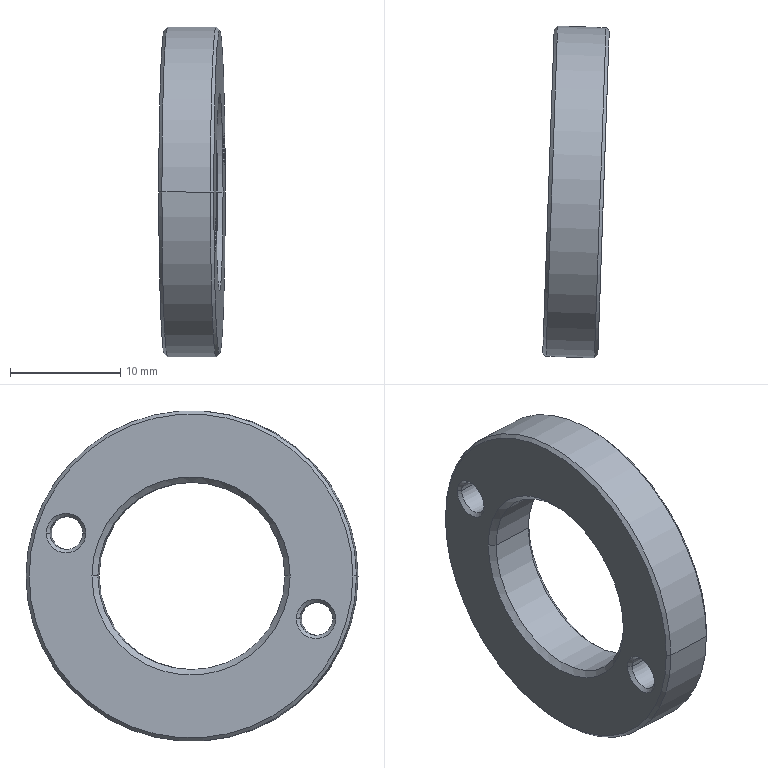Part | SolidWorks | features BaseBody 1 | 1 solid | 22 faces | box 6.032 x 30.136 x 30 mm | volume 2306 mm3 | cone 12 | cylinder 8 | plane 2 | commonest cylinder face diameters 3 x4 17 x2 30 x2
STEP:
#1=CARTESIAN_POINT('',(719.231,30.003,4.092));
#2=VERTEX_POINT('',#1);
#3=CARTESIAN_POINT('',(719.83,46.992,4.092));
#4=VERTEX_POINT('',#3);
#5=CARTESIAN_POINT('',(719.531,38.498,4.092));
#6=DIRECTION('',(0.9994,-0.0352,-0.000000013));
#7=DIRECTION('',(0.000000013,-0.000000004,1.));
#8=AXIS2_PLACEMENT_3D('',#5,#6,#7);
#9=CIRCLE('',#8,8.5);
#10=EDGE_CURVE('',#2,#4,#9,.T.);
#11=ORIENTED_EDGE('',*,*,#10,.F.);
#12=CARTESIAN_POINT('',(719.713,29.486,4.092));
#13=VERTEX_POINT('',#12);
#14=CARTESIAN_POINT('',(719.713,29.486,4.092));
#15=DIRECTION('',(0.6818,-0.7316,-0.000000009));
#16=VECTOR('',#15,1000.);
#17=LINE('',#14,#16);
#18=EDGE_CURVE('',#2,#13,#17,.T.);
#19=ORIENTED_EDGE('',*,*,#18,.T.);
#20=CARTESIAN_POINT('',(720.347,47.475,4.092));
#21=VERTEX_POINT('',#20);
#22=CARTESIAN_POINT('',(720.03,38.48,4.092));
#23=DIRECTION('',(0.9994,-0.0352,-0.000000013));
#24=DIRECTION('',(0.0352,0.9994,0.));
#25=AXIS2_PLACEMENT_3D('',#22,#23,#24);
#26=CIRCLE('',#25,9.);
#27=EDGE_CURVE('',#13,#21,#26,.T.);
#28=ORIENTED_EDGE('',*,*,#27,.T.);
#29=CARTESIAN_POINT('',(720.347,47.475,4.092));
#30=DIRECTION('',(0.7316,0.6818,-0.000000009));
#31=VECTOR('',#30,1000.);
#32=LINE('',#29,#31);
#33=EDGE_CURVE('',#4,#21,#32,.T.);
#34=ORIENTED_EDGE('',*,*,#33,.F.);
#35=EDGE_LOOP('',(#11,#19,#28,#34));
#36=FACE_OUTER_BOUND('',#35,.T.);
#37=CARTESIAN_POINT('',(720.03,38.48,4.092));
#38=DIRECTION('',(0.9994,-0.0352,-0.000000013));
#39=DIRECTION('',(0.0352,0.9994,0.));
#40=AXIS2_PLACEMENT_3D('',#37,#38,#39);
#41=CONICAL_SURFACE('',#40,9.,0.7854);
#42=ADVANCED_FACE('',(#36),#41,.F.);
#43=CARTESIAN_POINT('',(720.377,48.325,7.984));
#44=VERTEX_POINT('',#43);
#45=CARTESIAN_POINT('',(720.483,51.323,7.984));
#46=VERTEX_POINT('',#45);
#47=CARTESIAN_POINT('',(720.43,49.824,7.984));
#48=DIRECTION('',(0.9994,-0.0352,-0.000000013));
#49=DIRECTION('',(-0.0352,-0.9994,0.));
#50=AXIS2_PLACEMENT_3D('',#47,#48,#49);
#51=CIRCLE('',#50,1.5);
#52=EDGE_CURVE('',#44,#46,#51,.T.);
#53=ORIENTED_EDGE('',*,*,#52,.T.);
#54=CARTESIAN_POINT('',(715.786,51.489,7.984));
#55=VERTEX_POINT('',#54);
#56=CARTESIAN_POINT('',(715.486,51.499,7.984));
#57=DIRECTION('',(-0.9994,0.0352,0.000000013));
#58=VECTOR('',#57,1000.);
#59=LINE('',#56,#58);
#60=EDGE_CURVE('',#46,#55,#59,.T.);
#61=ORIENTED_EDGE('',*,*,#60,.T.);
#62=CARTESIAN_POINT('',(715.68,48.491,7.984));
#63=VERTEX_POINT('',#62);
#64=CARTESIAN_POINT('',(715.733,49.99,7.984));
#65=DIRECTION('',(0.9994,-0.0352,-0.000000013));
#66=DIRECTION('',(-0.0352,-0.9994,0.));
#67=AXIS2_PLACEMENT_3D('',#64,#65,#66);
#68=CIRCLE('',#67,1.5);
#69=EDGE_CURVE('',#63,#55,#68,.T.);
#70=ORIENTED_EDGE('',*,*,#69,.F.);
#71=CARTESIAN_POINT('',(715.38,48.501,7.984));
#72=DIRECTION('',(-0.9994,0.0352,0.000000013));
#73=VECTOR('',#72,1000.);
#74=LINE('',#71,#73);
#75=EDGE_CURVE('',#44,#63,#74,.T.);
#76=ORIENTED_EDGE('',*,*,#75,.F.);
#77=EDGE_LOOP('',(#53,#61,#70,#76));
#78=FACE_OUTER_BOUND('',#77,.T.);
#79=CARTESIAN_POINT('',(715.433,50.,7.984));
#80=DIRECTION('',(-0.9994,0.0352,0.000000013));
#81=DIRECTION('',(-0.0352,-0.9994,0.));
#82=AXIS2_PLACEMENT_3D('',#79,#80,#81);
#83=CYLINDRICAL_SURFACE('',#82,1.5);
#84=ADVANCED_FACE('',(#78),#83,.F.);
#85=CARTESIAN_POINT('',(719.578,25.637,0.1995));
#86=VERTEX_POINT('',#85);
#87=CARTESIAN_POINT('',(719.684,28.635,0.1995));
#88=VERTEX_POINT('',#87);
#89=CARTESIAN_POINT('',(719.631,27.136,0.1995));
#90=DIRECTION('',(0.9994,-0.0352,-0.000000013));
#91=DIRECTION('',(-0.0352,-0.9994,0.));
#92=AXIS2_PLACEMENT_3D('',#89,#90,#91);
#93=CIRCLE('',#92,1.5);
#94=EDGE_CURVE('',#86,#88,#93,.T.);
#95=ORIENTED_EDGE('',*,*,#94,.T.);
#96=CARTESIAN_POINT('',(714.986,28.8,0.1995));
#97=VERTEX_POINT('',#96);
#98=CARTESIAN_POINT('',(714.687,28.811,0.1995));
#99=DIRECTION('',(-0.9994,0.0352,0.000000013));
#100=VECTOR('',#99,1000.);
#101=LINE('',#98,#100);
#102=EDGE_CURVE('',#88,#97,#101,.T.);
#103=ORIENTED_EDGE('',*,*,#102,.T.);
#104=CARTESIAN_POINT('',(714.881,25.802,0.1995));
#105=VERTEX_POINT('',#104);
#106=CARTESIAN_POINT('',(714.934,27.301,0.1995));
#107=DIRECTION('',(0.9994,-0.0352,-0.000000013));
#108=DIRECTION('',(-0.0352,-0.9994,0.));
#109=AXIS2_PLACEMENT_3D('',#106,#107,#108);
#110=CIRCLE('',#109,1.5);
#111=EDGE_CURVE('',#105,#97,#110,.T.);
#112=ORIENTED_EDGE('',*,*,#111,.F.);
#113=CARTESIAN_POINT('',(714.581,25.813,0.1995));
#114=DIRECTION('',(-0.9994,0.0352,0.000000013));
#115=VECTOR('',#114,1000.);
#116=LINE('',#113,#115);
#117=EDGE_CURVE('',#86,#105,#116,.T.);
#118=ORIENTED_EDGE('',*,*,#117,.F.);
#119=EDGE_LOOP('',(#95,#103,#112,#118));
#120=FACE_OUTER_BOUND('',#119,.T.);
#121=CARTESIAN_POINT('',(714.634,27.312,0.1995));
#122=DIRECTION('',(-0.9994,0.0352,0.000000013));
#123=DIRECTION('',(-0.0352,-0.9994,0.));
#124=AXIS2_PLACEMENT_3D('',#121,#122,#123);
#125=CYLINDRICAL_SURFACE('',#124,1.5);
#126=ADVANCED_FACE('',(#120),#125,.F.);
#127=CARTESIAN_POINT('',(719.513,23.789,4.092));
#128=VERTEX_POINT('',#127);
#129=CARTESIAN_POINT('',(720.548,53.171,4.092));
#130=VERTEX_POINT('',#129);
#131=CARTESIAN_POINT('',(720.03,38.48,4.092));
#132=DIRECTION('',(-0.9994,0.0352,0.000000013));
#133=DIRECTION('',(-0.0352,-0.9994,0.));
#134=AXIS2_PLACEMENT_3D('',#131,#132,#133);
#135=CIRCLE('',#134,14.7);
#136=EDGE_CURVE('',#128,#130,#135,.T.);
#137=ORIENTED_EDGE('',*,*,#136,.T.);
#138=CARTESIAN_POINT('',(720.259,53.481,4.092));
#139=VERTEX_POINT('',#138);
#140=CARTESIAN_POINT('',(720.259,53.481,4.092));
#141=DIRECTION('',(-0.6818,0.7316,0.000000009));
#142=VECTOR('',#141,1000.);
#143=LINE('',#140,#142);
#144=EDGE_CURVE('',#130,#139,#143,.T.);
#145=ORIENTED_EDGE('',*,*,#144,.T.);
#146=CARTESIAN_POINT('',(719.202,23.5,4.092));
#147=VERTEX_POINT('',#146);
#148=CARTESIAN_POINT('',(719.731,38.491,4.092));
#149=DIRECTION('',(0.9994,-0.0352,-0.000000013));
#150=DIRECTION('',(0.000000013,-0.000000004,1.));
#151=AXIS2_PLACEMENT_3D('',#148,#149,#150);
#152=CIRCLE('',#151,15.);
#153=EDGE_CURVE('',#139,#147,#152,.T.);
#154=ORIENTED_EDGE('',*,*,#153,.T.);
#155=CARTESIAN_POINT('',(719.202,23.5,4.092));
#156=DIRECTION('',(-0.7316,-0.6818,0.000000009));
#157=VECTOR('',#156,1000.);
#158=LINE('',#155,#157);
#159=EDGE_CURVE('',#128,#147,#158,.T.);
#160=ORIENTED_EDGE('',*,*,#159,.F.);
#161=EDGE_LOOP('',(#137,#145,#154,#160));
#162=FACE_OUTER_BOUND('',#161,.T.);
#163=CARTESIAN_POINT('',(719.731,38.491,4.092));
#164=DIRECTION('',(-0.9994,0.0352,0.000000013));
#165=DIRECTION('',(-0.0352,-0.9994,0.));
#166=AXIS2_PLACEMENT_3D('',#163,#164,#165);
#167=CONICAL_SURFACE('',#166,15.,0.7854);
#168=ADVANCED_FACE('',(#162),#167,.T.);
#169=CARTESIAN_POINT('',(715.234,30.144,4.092));
#170=VERTEX_POINT('',#169);
#171=CARTESIAN_POINT('',(715.832,47.133,4.092));
#172=VERTEX_POINT('',#171);
#173=CARTESIAN_POINT('',(715.533,38.639,4.092));
#174=DIRECTION('',(0.9994,-0.0352,-0.000000013));
#175=DIRECTION('',(0.0352,0.9994,0.));
#176=AXIS2_PLACEMENT_3D('',#173,#174,#175);
#177=CIRCLE('',#176,8.5);
#178=EDGE_CURVE('',#170,#172,#177,.T.);
#179=ORIENTED_EDGE('',*,*,#178,.F.);
#180=CARTESIAN_POINT('',(717.233,30.073,4.092));
#181=DIRECTION('',(0.9994,-0.0352,-0.000000013));
#182=VECTOR('',#181,1000.);
#183=LINE('',#180,#182);
#184=EDGE_CURVE('',#170,#2,#183,.T.);
#185=ORIENTED_EDGE('',*,*,#184,.T.);
#186=ORIENTED_EDGE('',*,*,#10,.T.);
#187=CARTESIAN_POINT('',(717.831,47.063,4.092));
#188=DIRECTION('',(0.9994,-0.0352,-0.000000013));
#189=VECTOR('',#188,1000.);
#190=LINE('',#187,#189);
#191=EDGE_CURVE('',#172,#4,#190,.T.);
#192=ORIENTED_EDGE('',*,*,#191,.F.);
#193=EDGE_LOOP('',(#179,#185,#186,#192));
#194=FACE_OUTER_BOUND('',#193,.T.);
#195=CARTESIAN_POINT('',(717.532,38.568,4.092));
#196=DIRECTION('',(0.9994,-0.0352,-0.000000013));
#197=DIRECTION('',(0.0352,0.9994,0.));
#198=AXIS2_PLACEMENT_3D('',#195,#196,#197);
#199=CYLINDRICAL_SURFACE('',#198,8.5);
#200=ADVANCED_FACE('',(#194),#199,.F.);
#201=ORIENTED_EDGE('',*,*,#69,.T.);
#202=CARTESIAN_POINT('',(715.496,51.799,7.984));
#203=VERTEX_POINT('',#202);
#204=CARTESIAN_POINT('',(715.496,51.799,7.984));
#205=DIRECTION('',(-0.6818,0.7316,0.000000009));
#206=VECTOR('',#205,1000.);
#207=LINE('',#204,#206);
#208=EDGE_CURVE('',#55,#203,#207,.T.);
#209=ORIENTED_EDGE('',*,*,#208,.T.);
#210=CARTESIAN_POINT('',(715.37,48.201,7.984));
#211=VERTEX_POINT('',#210);
#212=CARTESIAN_POINT('',(715.433,50.,7.984));
#213=DIRECTION('',(0.9994,-0.0352,-0.000000013));
#214=DIRECTION('',(-0.0352,-0.9994,0.));
#215=AXIS2_PLACEMENT_3D('',#212,#213,#214);
#216=CIRCLE('',#215,1.8);
#217=EDGE_CURVE('',#211,#203,#216,.T.);
#218=ORIENTED_EDGE('',*,*,#217,.F.);
#219=CARTESIAN_POINT('',(715.37,48.201,7.984));
#220=DIRECTION('',(-0.7316,-0.6818,0.000000009));
#221=VECTOR('',#220,1000.);
#222=LINE('',#219,#221);
#223=EDGE_CURVE('',#63,#211,#222,.T.);
#224=ORIENTED_EDGE('',*,*,#223,.F.);
#225=EDGE_LOOP('',(#201,#209,#218,#224));
#226=FACE_OUTER_BOUND('',#225,.T.);
#227=CARTESIAN_POINT('',(715.433,50.,7.984));
#228=DIRECTION('',(-0.9994,0.0352,0.000000013));
#229=DIRECTION('',(-0.0352,-0.9994,0.));
#230=AXIS2_PLACEMENT_3D('',#227,#228,#229);
#231=CONICAL_SURFACE('',#230,1.8,0.7854);
#232=ADVANCED_FACE('',(#226),#231,.F.);
#233=ORIENTED_EDGE('',*,*,#111,.T.);
#234=CARTESIAN_POINT('',(714.697,29.111,0.1995));
#235=VERTEX_POINT('',#234);
#236=CARTESIAN_POINT('',(714.697,29.111,0.1995));
#237=DIRECTION('',(-0.6818,0.7316,0.000000009));
#238=VECTOR('',#237,1000.);
#239=LINE('',#236,#238);
#240=EDGE_CURVE('',#97,#235,#239,.T.);
#241=ORIENTED_EDGE('',*,*,#240,.T.);
#242=CARTESIAN_POINT('',(714.57,25.513,0.1995));
#243=VERTEX_POINT('',#242);
#244=CARTESIAN_POINT('',(714.634,27.312,0.1995));
#245=DIRECTION('',(0.9994,-0.0352,-0.000000013));
#246=DIRECTION('',(-0.0352,-0.9994,0.));
#247=AXIS2_PLACEMENT_3D('',#244,#245,#246);
#248=CIRCLE('',#247,1.8);
#249=EDGE_CURVE('',#243,#235,#248,.T.);
#250=ORIENTED_EDGE('',*,*,#249,.F.);
#251=CARTESIAN_POINT('',(714.57,25.513,0.1995));
#252=DIRECTION('',(-0.7316,-0.6818,0.000000009));
#253=VECTOR('',#252,1000.);
#254=LINE('',#251,#253);
#255=EDGE_CURVE('',#105,#243,#254,.T.);
#256=ORIENTED_EDGE('',*,*,#255,.F.);
#257=EDGE_LOOP('',(#233,#241,#250,#256));
#258=FACE_OUTER_BOUND('',#257,.T.);
#259=CARTESIAN_POINT('',(714.634,27.312,0.1995));
#260=DIRECTION('',(-0.9994,0.0352,0.000000013));
#261=DIRECTION('',(-0.0352,-0.9994,0.));
#262=AXIS2_PLACEMENT_3D('',#259,#260,#261);
#263=CONICAL_SURFACE('',#262,1.8,0.7854);
#264=ADVANCED_FACE('',(#258),#263,.F.);
#265=CARTESIAN_POINT('',(715.861,53.636,4.092));
#266=VERTEX_POINT('',#265);
#267=CARTESIAN_POINT('',(714.805,23.655,4.092));
#268=VERTEX_POINT('',#267);
#269=CARTESIAN_POINT('',(715.333,38.646,4.092));
#270=DIRECTION('',(0.9994,-0.0352,-0.000000013));
#271=DIRECTION('',(0.0352,0.9994,0.));
#272=AXIS2_PLACEMENT_3D('',#269,#270,#271);
#273=CIRCLE('',#272,15.);
#274=EDGE_CURVE('',#266,#268,#273,.T.);
#275=ORIENTED_EDGE('',*,*,#274,.T.);
#276=CARTESIAN_POINT('',(719.502,23.489,4.092));
#277=DIRECTION('',(0.9994,-0.0352,-0.000000013));
#278=VECTOR('',#277,1000.);
#279=LINE('',#276,#278);
#280=EDGE_CURVE('',#268,#147,#279,.T.);
#281=ORIENTED_EDGE('',*,*,#280,.T.);
#282=ORIENTED_EDGE('',*,*,#153,.F.);
#283=CARTESIAN_POINT('',(720.558,53.471,4.092));
#284=DIRECTION('',(0.9994,-0.0352,-0.000000013));
#285=VECTOR('',#284,1000.);
#286=LINE('',#283,#285);
#287=EDGE_CURVE('',#266,#139,#286,.T.);
#288=ORIENTED_EDGE('',*,*,#287,.F.);
#289=EDGE_LOOP('',(#275,#281,#282,#288));
#290=FACE_OUTER_BOUND('',#289,.T.);
#291=CARTESIAN_POINT('',(720.03,38.48,4.092));
#292=DIRECTION('',(0.9994,-0.0352,-0.000000013));
#293=DIRECTION('',(0.0352,0.9994,0.));
#294=AXIS2_PLACEMENT_3D('',#291,#292,#293);
#295=CYLINDRICAL_SURFACE('',#294,15.);
#296=ADVANCED_FACE('',(#290),#295,.T.);
#297=ORIENTED_EDGE('',*,*,#178,.T.);
#298=CARTESIAN_POINT('',(715.35,47.651,4.092));
#299=VERTEX_POINT('',#298);
#300=CARTESIAN_POINT('',(715.35,47.651,4.092));
#301=DIRECTION('',(-0.6818,0.7316,0.000000009));
#302=VECTOR('',#301,1000.);
#303=LINE('',#300,#302);
#304=EDGE_CURVE('',#172,#299,#303,.T.);
#305=ORIENTED_EDGE('',*,*,#304,.T.);
#306=CARTESIAN_POINT('',(714.717,29.662,4.092));
#307=VERTEX_POINT('',#306);
#308=CARTESIAN_POINT('',(715.033,38.656,4.092));
#309=DIRECTION('',(0.9994,-0.0352,-0.000000013));
#310=DIRECTION('',(-0.0352,-0.9994,0.));
#311=AXIS2_PLACEMENT_3D('',#308,#309,#310);
#312=CIRCLE('',#311,9.);
#313=EDGE_CURVE('',#307,#299,#312,.T.);
#314=ORIENTED_EDGE('',*,*,#313,.F.);
#315=CARTESIAN_POINT('',(714.717,29.662,4.092));
#316=DIRECTION('',(-0.7316,-0.6818,0.000000009));
#317=VECTOR('',#316,1000.);
#318=LINE('',#315,#317);
#319=EDGE_CURVE('',#170,#307,#318,.T.);
#320=ORIENTED_EDGE('',*,*,#319,.F.);
#321=EDGE_LOOP('',(#297,#305,#314,#320));
#322=FACE_OUTER_BOUND('',#321,.T.);
#323=CARTESIAN_POINT('',(715.033,38.656,4.092));
#324=DIRECTION('',(-0.9994,0.0352,0.000000013));
#325=DIRECTION('',(-0.0352,-0.9994,0.));
#326=AXIS2_PLACEMENT_3D('',#323,#324,#325);
#327=CONICAL_SURFACE('',#326,9.,0.7854);
#328=ADVANCED_FACE('',(#322),#327,.F.);
#329=CARTESIAN_POINT('',(714.516,23.965,4.092));
#330=VERTEX_POINT('',#329);
#331=CARTESIAN_POINT('',(715.551,53.347,4.092));
#332=VERTEX_POINT('',#331);
#333=CARTESIAN_POINT('',(715.033,38.656,4.092));
#334=DIRECTION('',(-0.9994,0.0352,0.000000013));
#335=DIRECTION('',(0.0352,0.9994,0.));
#336=AXIS2_PLACEMENT_3D('',#333,#334,#335);
#337=CIRCLE('',#336,14.7);
#338=EDGE_CURVE('',#330,#332,#337,.T.);
#339=ORIENTED_EDGE('',*,*,#338,.F.);
#340=CARTESIAN_POINT('',(714.805,23.655,4.092));
#341=DIRECTION('',(0.6818,-0.7316,-0.000000009));
#342=VECTOR('',#341,1000.);
#343=LINE('',#340,#342);
#344=EDGE_CURVE('',#330,#268,#343,.T.);
#345=ORIENTED_EDGE('',*,*,#344,.T.);
#346=ORIENTED_EDGE('',*,*,#274,.F.);
#347=CARTESIAN_POINT('',(715.861,53.636,4.092));
#348=DIRECTION('',(0.7316,0.6818,-0.000000009));
#349=VECTOR('',#348,1000.);
#350=LINE('',#347,#349);
#351=EDGE_CURVE('',#332,#266,#350,.T.);
#352=ORIENTED_EDGE('',*,*,#351,.F.);
#353=EDGE_LOOP('',(#339,#345,#346,#352));
#354=FACE_OUTER_BOUND('',#353,.T.);
#355=CARTESIAN_POINT('',(715.333,38.646,4.092));
#356=DIRECTION('',(0.9994,-0.0352,-0.000000013));
#357=DIRECTION('',(0.0352,0.9994,0.));
#358=AXIS2_PLACEMENT_3D('',#355,#356,#357);
#359=CONICAL_SURFACE('',#358,15.,0.7854);
#360=ADVANCED_FACE('',(#354),#359,.T.);
#361=CARTESIAN_POINT('',(720.03,38.48,4.092));
#362=DIRECTION('',(0.9994,-0.0352,-0.000000013));
#363=DIRECTION('',(0.0352,0.9994,0.));
#364=AXIS2_PLACEMENT_3D('',#361,#362,#363);
#365=CIRCLE('',#364,9.);
#366=EDGE_CURVE('',#21,#13,#365,.T.);
#367=ORIENTED_EDGE('',*,*,#366,.F.);
#368=ORIENTED_EDGE('',*,*,#27,.F.);
#369=EDGE_LOOP('',(#367,#368));
#370=FACE_BOUND('',#369,.T.);
#371=ORIENTED_EDGE('',*,*,#52,.F.);
#372=CARTESIAN_POINT('',(720.43,49.824,7.984));
#373=DIRECTION('',(0.9994,-0.0352,-0.000000013));
#374=DIRECTION('',(-0.0352,-0.9994,0.));
#375=AXIS2_PLACEMENT_3D('',#372,#373,#374);
#376=CIRCLE('',#375,1.5);
#377=EDGE_CURVE('',#46,#44,#376,.T.);
#378=ORIENTED_EDGE('',*,*,#377,.F.);
#379=EDGE_LOOP('',(#371,#378));
#380=FACE_BOUND('',#379,.T.);
#381=ORIENTED_EDGE('',*,*,#94,.F.);
#382=CARTESIAN_POINT('',(719.631,27.136,0.1995));
#383=DIRECTION('',(0.9994,-0.0352,-0.000000013));
#384=DIRECTION('',(-0.0352,-0.9994,0.));
#385=AXIS2_PLACEMENT_3D('',#382,#383,#384);
#386=CIRCLE('',#385,1.5);
#387=EDGE_CURVE('',#88,#86,#386,.T.);
#388=ORIENTED_EDGE('',*,*,#387,.F.);
#389=EDGE_LOOP('',(#381,#388));
#390=FACE_BOUND('',#389,.T.);
#391=ORIENTED_EDGE('',*,*,#136,.F.);
#392=CARTESIAN_POINT('',(720.03,38.48,4.092));
#393=DIRECTION('',(-0.9994,0.0352,0.000000013));
#394=DIRECTION('',(-0.0352,-0.9994,0.));
#395=AXIS2_PLACEMENT_3D('',#392,#393,#394);
#396=CIRCLE('',#395,14.7);
#397=EDGE_CURVE('',#130,#128,#396,.T.);
#398=ORIENTED_EDGE('',*,*,#397,.F.);
#399=EDGE_LOOP('',(#391,#398));
#400=FACE_OUTER_BOUND('',#399,.T.);
#401=CARTESIAN_POINT('',(720.03,38.48,4.092));
#402=DIRECTION('',(-0.9994,0.0352,0.000000013));
#403=DIRECTION('',(-0.0352,-0.9994,0.));
#404=AXIS2_PLACEMENT_3D('',#401,#402,#403);
#405=PLANE('',#404);
#406=ADVANCED_FACE('',(#370,#380,#390,#400),#405,.F.);
#407=ORIENTED_EDGE('',*,*,#18,.F.);
#408=CARTESIAN_POINT('',(719.531,38.498,4.092));
#409=DIRECTION('',(0.9994,-0.0352,-0.000000013));
#410=DIRECTION('',(0.000000013,-0.000000004,1.));
#411=AXIS2_PLACEMENT_3D('',#408,#409,#410);
#412=CIRCLE('',#411,8.5);
#413=EDGE_CURVE('',#4,#2,#412,.T.);
#414=ORIENTED_EDGE('',*,*,#413,.F.);
#415=ORIENTED_EDGE('',*,*,#33,.T.);
#416=ORIENTED_EDGE('',*,*,#366,.T.);
#417=EDGE_LOOP('',(#407,#414,#415,#416));
#418=FACE_OUTER_BOUND('',#417,.T.);
#419=CARTESIAN_POINT('',(720.03,38.48,4.092));
#420=DIRECTION('',(0.9994,-0.0352,-0.000000013));
#421=DIRECTION('',(0.0352,0.9994,0.));
#422=AXIS2_PLACEMENT_3D('',#419,#420,#421);
#423=CONICAL_SURFACE('',#422,9.,0.7854);
#424=ADVANCED_FACE('',(#418),#423,.F.);
#425=ORIENTED_EDGE('',*,*,#60,.F.);
#426=ORIENTED_EDGE('',*,*,#377,.T.);
#427=ORIENTED_EDGE('',*,*,#75,.T.);
#428=CARTESIAN_POINT('',(715.733,49.99,7.984));
#429=DIRECTION('',(0.9994,-0.0352,-0.000000013));
#430=DIRECTION('',(-0.0352,-0.9994,0.));
#431=AXIS2_PLACEMENT_3D('',#428,#429,#430);
#432=CIRCLE('',#431,1.5);
#433=EDGE_CURVE('',#55,#63,#432,.T.);
#434=ORIENTED_EDGE('',*,*,#433,.F.);
#435=EDGE_LOOP('',(#425,#426,#427,#434));
#436=FACE_OUTER_BOUND('',#435,.T.);
#437=CARTESIAN_POINT('',(715.433,50.,7.984));
#438=DIRECTION('',(-0.9994,0.0352,0.000000013));
#439=DIRECTION('',(-0.0352,-0.9994,0.));
#440=AXIS2_PLACEMENT_3D('',#437,#438,#439);
#441=CYLINDRICAL_SURFACE('',#440,1.5);
#442=ADVANCED_FACE('',(#436),#441,.F.);
#443=ORIENTED_EDGE('',*,*,#102,.F.);
#444=ORIENTED_EDGE('',*,*,#387,.T.);
#445=ORIENTED_EDGE('',*,*,#117,.T.);
#446=CARTESIAN_POINT('',(714.934,27.301,0.1995));
#447=DIRECTION('',(0.9994,-0.0352,-0.000000013));
#448=DIRECTION('',(-0.0352,-0.9994,0.));
#449=AXIS2_PLACEMENT_3D('',#446,#447,#448);
#450=CIRCLE('',#449,1.5);
#451=EDGE_CURVE('',#97,#105,#450,.T.);
#452=ORIENTED_EDGE('',*,*,#451,.F.);
#453=EDGE_LOOP('',(#443,#444,#445,#452));
#454=FACE_OUTER_BOUND('',#453,.T.);
#455=CARTESIAN_POINT('',(714.634,27.312,0.1995));
#456=DIRECTION('',(-0.9994,0.0352,0.000000013));
#457=DIRECTION('',(-0.0352,-0.9994,0.));
#458=AXIS2_PLACEMENT_3D('',#455,#456,#457);
#459=CYLINDRICAL_SURFACE('',#458,1.5);
#460=ADVANCED_FACE('',(#454),#459,.F.);
#461=ORIENTED_EDGE('',*,*,#144,.F.);
#462=ORIENTED_EDGE('',*,*,#397,.T.);
#463=ORIENTED_EDGE('',*,*,#159,.T.);
#464=CARTESIAN_POINT('',(719.731,38.491,4.092));
#465=DIRECTION('',(0.9994,-0.0352,-0.000000013));
#466=DIRECTION('',(0.000000013,-0.000000004,1.));
#467=AXIS2_PLACEMENT_3D('',#464,#465,#466);
#468=CIRCLE('',#467,15.);
#469=EDGE_CURVE('',#147,#139,#468,.T.);
#470=ORIENTED_EDGE('',*,*,#469,.T.);
#471=EDGE_LOOP('',(#461,#462,#463,#470));
#472=FACE_OUTER_BOUND('',#471,.T.);
#473=CARTESIAN_POINT('',(719.731,38.491,4.092));
#474=DIRECTION('',(-0.9994,0.0352,0.000000013));
#475=DIRECTION('',(-0.0352,-0.9994,0.));
#476=AXIS2_PLACEMENT_3D('',#473,#474,#475);
#477=CONICAL_SURFACE('',#476,15.,0.7854);
#478=ADVANCED_FACE('',(#472),#477,.T.);
#479=ORIENTED_EDGE('',*,*,#184,.F.);
#480=CARTESIAN_POINT('',(715.533,38.639,4.092));
#481=DIRECTION('',(0.9994,-0.0352,-0.000000013));
#482=DIRECTION('',(0.0352,0.9994,0.));
#483=AXIS2_PLACEMENT_3D('',#480,#481,#482);
#484=CIRCLE('',#483,8.5);
#485=EDGE_CURVE('',#172,#170,#484,.T.);
#486=ORIENTED_EDGE('',*,*,#485,.F.);
#487=ORIENTED_EDGE('',*,*,#191,.T.);
#488=ORIENTED_EDGE('',*,*,#413,.T.);
#489=EDGE_LOOP('',(#479,#486,#487,#488));
#490=FACE_OUTER_BOUND('',#489,.T.);
#491=CARTESIAN_POINT('',(717.532,38.568,4.092));
#492=DIRECTION('',(0.9994,-0.0352,-0.000000013));
#493=DIRECTION('',(0.0352,0.9994,0.));
#494=AXIS2_PLACEMENT_3D('',#491,#492,#493);
#495=CYLINDRICAL_SURFACE('',#494,8.5);
#496=ADVANCED_FACE('',(#490),#495,.F.);
#497=ORIENTED_EDGE('',*,*,#208,.F.);
#498=ORIENTED_EDGE('',*,*,#433,.T.);
#499=ORIENTED_EDGE('',*,*,#223,.T.);
#500=CARTESIAN_POINT('',(715.433,50.,7.984));
#501=DIRECTION('',(0.9994,-0.0352,-0.000000013));
#502=DIRECTION('',(-0.0352,-0.9994,0.));
#503=AXIS2_PLACEMENT_3D('',#500,#501,#502);
#504=CIRCLE('',#503,1.8);
#505=EDGE_CURVE('',#203,#211,#504,.T.);
#506=ORIENTED_EDGE('',*,*,#505,.F.);
#507=EDGE_LOOP('',(#497,#498,#499,#506));
#508=FACE_OUTER_BOUND('',#507,.T.);
#509=CARTESIAN_POINT('',(715.433,50.,7.984));
#510=DIRECTION('',(-0.9994,0.0352,0.000000013));
#511=DIRECTION('',(-0.0352,-0.9994,0.));
#512=AXIS2_PLACEMENT_3D('',#509,#510,#511);
#513=CONICAL_SURFACE('',#512,1.8,0.7854);
#514=ADVANCED_FACE('',(#508),#513,.F.);
#515=ORIENTED_EDGE('',*,*,#240,.F.);
#516=ORIENTED_EDGE('',*,*,#451,.T.);
#517=ORIENTED_EDGE('',*,*,#255,.T.);
#518=CARTESIAN_POINT('',(714.634,27.312,0.1995));
#519=DIRECTION('',(0.9994,-0.0352,-0.000000013));
#520=DIRECTION('',(-0.0352,-0.9994,0.));
#521=AXIS2_PLACEMENT_3D('',#518,#519,#520);
#522=CIRCLE('',#521,1.8);
#523=EDGE_CURVE('',#235,#243,#522,.T.);
#524=ORIENTED_EDGE('',*,*,#523,.F.);
#525=EDGE_LOOP('',(#515,#516,#517,#524));
#526=FACE_OUTER_BOUND('',#525,.T.);
#527=CARTESIAN_POINT('',(714.634,27.312,0.1995));
#528=DIRECTION('',(-0.9994,0.0352,0.000000013));
#529=DIRECTION('',(-0.0352,-0.9994,0.));
#530=AXIS2_PLACEMENT_3D('',#527,#528,#529);
#531=CONICAL_SURFACE('',#530,1.8,0.7854);
#532=ADVANCED_FACE('',(#526),#531,.F.);
#533=ORIENTED_EDGE('',*,*,#280,.F.);
#534=CARTESIAN_POINT('',(715.333,38.646,4.092));
#535=DIRECTION('',(0.9994,-0.0352,-0.000000013));
#536=DIRECTION('',(0.0352,0.9994,0.));
#537=AXIS2_PLACEMENT_3D('',#534,#535,#536);
#538=CIRCLE('',#537,15.);
#539=EDGE_CURVE('',#268,#266,#538,.T.);
#540=ORIENTED_EDGE('',*,*,#539,.T.);
#541=ORIENTED_EDGE('',*,*,#287,.T.);
#542=ORIENTED_EDGE('',*,*,#469,.F.);
#543=EDGE_LOOP('',(#533,#540,#541,#542));
#544=FACE_OUTER_BOUND('',#543,.T.);
#545=CARTESIAN_POINT('',(720.03,38.48,4.092));
#546=DIRECTION('',(0.9994,-0.0352,-0.000000013));
#547=DIRECTION('',(0.0352,0.9994,0.));
#548=AXIS2_PLACEMENT_3D('',#545,#546,#547);
#549=CYLINDRICAL_SURFACE('',#548,15.);
#550=ADVANCED_FACE('',(#544),#549,.T.);
#551=ORIENTED_EDGE('',*,*,#304,.F.);
#552=ORIENTED_EDGE('',*,*,#485,.T.);
#553=ORIENTED_EDGE('',*,*,#319,.T.);
#554=CARTESIAN_POINT('',(715.033,38.656,4.092));
#555=DIRECTION('',(0.9994,-0.0352,-0.000000013));
#556=DIRECTION('',(-0.0352,-0.9994,0.));
#557=AXIS2_PLACEMENT_3D('',#554,#555,#556);
#558=CIRCLE('',#557,9.);
#559=EDGE_CURVE('',#299,#307,#558,.T.);
#560=ORIENTED_EDGE('',*,*,#559,.F.);
#561=EDGE_LOOP('',(#551,#552,#553,#560));
#562=FACE_OUTER_BOUND('',#561,.T.);
#563=CARTESIAN_POINT('',(715.033,38.656,4.092));
#564=DIRECTION('',(-0.9994,0.0352,0.000000013));
#565=DIRECTION('',(-0.0352,-0.9994,0.));
#566=AXIS2_PLACEMENT_3D('',#563,#564,#565);
#567=CONICAL_SURFACE('',#566,9.,0.7854);
#568=ADVANCED_FACE('',(#562),#567,.F.);
#569=ORIENTED_EDGE('',*,*,#313,.T.);
#570=ORIENTED_EDGE('',*,*,#559,.T.);
#571=EDGE_LOOP('',(#569,#570));
#572=FACE_BOUND('',#571,.T.);
#573=ORIENTED_EDGE('',*,*,#217,.T.);
#574=ORIENTED_EDGE('',*,*,#505,.T.);
#575=EDGE_LOOP('',(#573,#574));
#576=FACE_BOUND('',#575,.T.);
#577=CARTESIAN_POINT('',(715.033,38.656,4.092));
#578=DIRECTION('',(-0.9994,0.0352,0.000000013));
#579=DIRECTION('',(0.0352,0.9994,0.));
#580=AXIS2_PLACEMENT_3D('',#577,#578,#579);
#581=CIRCLE('',#580,14.7);
#582=EDGE_CURVE('',#332,#330,#581,.T.);
#583=ORIENTED_EDGE('',*,*,#582,.T.);
#584=ORIENTED_EDGE('',*,*,#338,.T.);
#585=EDGE_LOOP('',(#583,#584));
#586=FACE_OUTER_BOUND('',#585,.T.);
#587=ORIENTED_EDGE('',*,*,#249,.T.);
#588=ORIENTED_EDGE('',*,*,#523,.T.);
#589=EDGE_LOOP('',(#587,#588));
#590=FACE_BOUND('',#589,.T.);
#591=CARTESIAN_POINT('',(715.033,38.656,4.092));
#592=DIRECTION('',(-0.9994,0.0352,0.000000013));
#593=DIRECTION('',(-0.0352,-0.9994,0.));
#594=AXIS2_PLACEMENT_3D('',#591,#592,#593);
#595=PLANE('',#594);
#596=ADVANCED_FACE('',(#572,#576,#586,#590),#595,.T.);
#597=ORIENTED_EDGE('',*,*,#344,.F.);
#598=ORIENTED_EDGE('',*,*,#582,.F.);
#599=ORIENTED_EDGE('',*,*,#351,.T.);
#600=ORIENTED_EDGE('',*,*,#539,.F.);
#601=EDGE_LOOP('',(#597,#598,#599,#600));
#602=FACE_OUTER_BOUND('',#601,.T.);
#603=CARTESIAN_POINT('',(715.333,38.646,4.092));
#604=DIRECTION('',(0.9994,-0.0352,-0.000000013));
#605=DIRECTION('',(0.0352,0.9994,0.));
#606=AXIS2_PLACEMENT_3D('',#603,#604,#605);
#607=CONICAL_SURFACE('',#606,15.,0.7854);
#608=ADVANCED_FACE('',(#602),#607,.T.);
#609=CLOSED_SHELL('',(#42,#84,#126,#168,#200,#232,#264,#296,#328,#360,#406,#424,#442,#460,#478,#496,#514,#532,#550,#568,#596,#608));
#610=MANIFOLD_SOLID_BREP('',#609);
#611=CARTESIAN_POINT('',(0.,0.,0.));
#612=DIRECTION('',(0.,0.,1.));
#613=DIRECTION('',(1.,0.,0.));
#614=AXIS2_PLACEMENT_3D('',#611,#612,#613);
#615=(LENGTH_UNIT()NAMED_UNIT(*)SI_UNIT(.MILLI.,.METRE.));
#616=UNCERTAINTY_MEASURE_WITH_UNIT(LENGTH_MEASURE(0.00001),#615,'','');
#617=(NAMED_UNIT(*)PLANE_ANGLE_UNIT()SI_UNIT($,.RADIAN.));
#618=(NAMED_UNIT(*)SI_UNIT($,.STERADIAN.)SOLID_ANGLE_UNIT());
#619=(GEOMETRIC_REPRESENTATION_CONTEXT(3)GLOBAL_UNCERTAINTY_ASSIGNED_CONTEXT((#616))GLOBAL_UNIT_ASSIGNED_CONTEXT((#615,#617,#618))REPRESENTATION_CONTEXT('',''));
#620=ADVANCED_BREP_SHAPE_REPRESENTATION('',(#610,#614),#619);